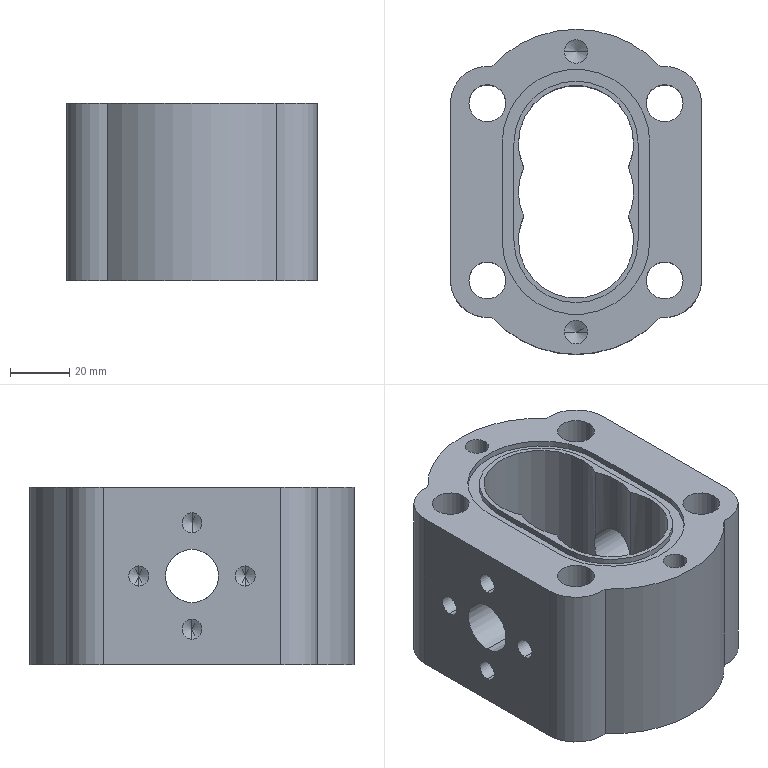Part | SolidWorks | features ICE 7, HoleWzd 3, MirrorPattern 3, Split 2, BlendCut 1, Extrusion 1, Fillet 1, MoveFace 1 | 1 solid | 94 faces | box 85 x 110 x 60 mm | volume 286652 mm3 | cylinder 58 | cone 20 | plane 16 | commonest cylinder face diameters 6.8 x16 39 x12 12.5 x8 8 x4 18 x4 25 x4